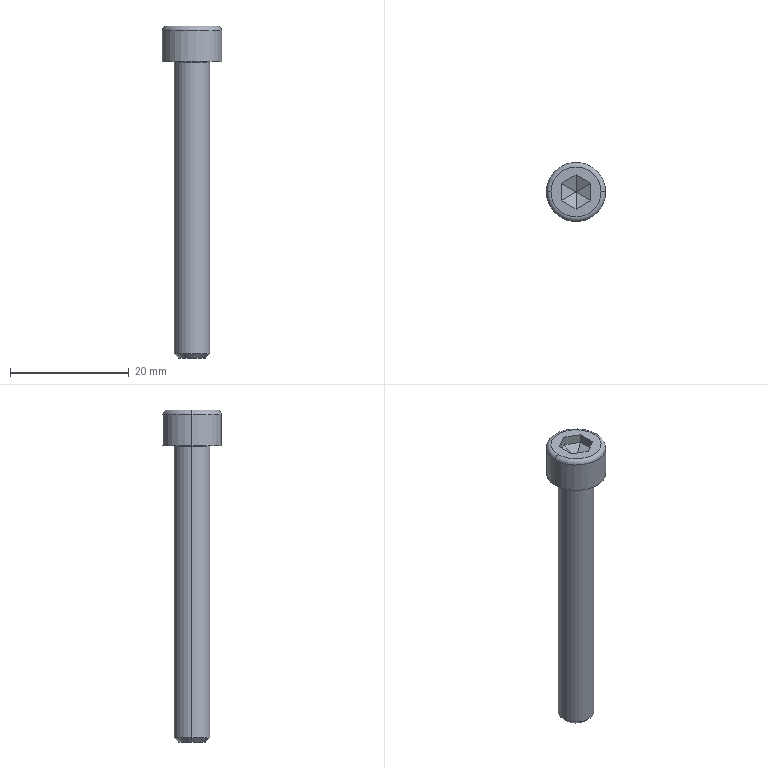Part | SolidWorks | features Chamfer 2, Fillet 2, ICE 2, Extrusion 1, RefAxis 1 | 1 solid | 26 faces | box 10 x 10 x 56 mm | volume 1832 mm3 | plane 16 | torus 4 | cylinder 4 | cone 2 | commonest cylinder face diameters 6 x2 10 x2
STEP:
#1=CARTESIAN_POINT('',(-3.1,0.,0.));
#2=VERTEX_POINT('',#1);
#3=CARTESIAN_POINT('',(3.1,0.,0.));
#4=VERTEX_POINT('',#3);
#5=CARTESIAN_POINT('',(0.,0.,0.));
#6=DIRECTION('',(0.,0.,1.));
#7=DIRECTION('',(1.,0.,0.));
#8=AXIS2_PLACEMENT_3D('',#5,#6,#7);
#9=CIRCLE('',#8,3.1);
#10=EDGE_CURVE('',#2,#4,#9,.T.);
#11=ORIENTED_EDGE('',*,*,#10,.F.);
#12=CARTESIAN_POINT('',(-3.,0.,-0.1));
#13=VERTEX_POINT('',#12);
#14=CARTESIAN_POINT('',(-3.1,0.,-0.1));
#15=DIRECTION('',(0.,1.,0.));
#16=DIRECTION('',(-1.,0.,0.));
#17=AXIS2_PLACEMENT_3D('',#14,#15,#16);
#18=CIRCLE('',#17,0.1);
#19=EDGE_CURVE('',#2,#13,#18,.T.);
#20=ORIENTED_EDGE('',*,*,#19,.T.);
#21=CARTESIAN_POINT('',(3.,0.,-0.1));
#22=VERTEX_POINT('',#21);
#23=CARTESIAN_POINT('',(0.,0.,-0.1));
#24=DIRECTION('',(0.,0.,-1.));
#25=DIRECTION('',(1.,0.,0.));
#26=AXIS2_PLACEMENT_3D('',#23,#24,#25);
#27=CIRCLE('',#26,3.);
#28=EDGE_CURVE('',#22,#13,#27,.T.);
#29=ORIENTED_EDGE('',*,*,#28,.F.);
#30=CARTESIAN_POINT('',(3.1,0.,-0.1));
#31=DIRECTION('',(0.,-1.,0.));
#32=DIRECTION('',(0.,0.,-1.));
#33=AXIS2_PLACEMENT_3D('',#30,#31,#32);
#34=CIRCLE('',#33,0.1);
#35=EDGE_CURVE('',#4,#22,#34,.T.);
#36=ORIENTED_EDGE('',*,*,#35,.F.);
#37=EDGE_LOOP('',(#11,#20,#29,#36));
#38=FACE_OUTER_BOUND('',#37,.T.);
#39=CARTESIAN_POINT('',(0.,0.,-0.1));
#40=DIRECTION('',(0.,0.,1.));
#41=DIRECTION('',(1.,0.,0.));
#42=AXIS2_PLACEMENT_3D('',#39,#40,#41);
#43=TOROIDAL_SURFACE('',#42,3.1,0.1);
#44=ADVANCED_FACE('',(#38),#43,.F.);
#45=CARTESIAN_POINT('',(-5.,0.,5.231));
#46=VERTEX_POINT('',#45);
#47=CARTESIAN_POINT('',(5.,0.,5.231));
#48=VERTEX_POINT('',#47);
#49=CARTESIAN_POINT('',(0.,0.,5.231));
#50=DIRECTION('',(0.,0.,-1.));
#51=DIRECTION('',(1.,0.,0.));
#52=AXIS2_PLACEMENT_3D('',#49,#50,#51);
#53=CIRCLE('',#52,5.);
#54=EDGE_CURVE('',#46,#48,#53,.T.);
#55=ORIENTED_EDGE('',*,*,#54,.F.);
#56=CARTESIAN_POINT('',(-4.231,0.,6.));
#57=VERTEX_POINT('',#56);
#58=CARTESIAN_POINT('',(-4.231,0.,5.231));
#59=DIRECTION('',(0.,1.,0.));
#60=DIRECTION('',(-1.,0.,0.));
#61=AXIS2_PLACEMENT_3D('',#58,#59,#60);
#62=CIRCLE('',#61,0.7692);
#63=EDGE_CURVE('',#46,#57,#62,.T.);
#64=ORIENTED_EDGE('',*,*,#63,.T.);
#65=CARTESIAN_POINT('',(4.231,0.,6.));
#66=VERTEX_POINT('',#65);
#67=CARTESIAN_POINT('',(0.,0.,6.));
#68=DIRECTION('',(0.,0.,1.));
#69=DIRECTION('',(1.,0.,0.));
#70=AXIS2_PLACEMENT_3D('',#67,#68,#69);
#71=CIRCLE('',#70,4.231);
#72=EDGE_CURVE('',#66,#57,#71,.T.);
#73=ORIENTED_EDGE('',*,*,#72,.F.);
#74=CARTESIAN_POINT('',(4.231,0.,5.231));
#75=DIRECTION('',(0.,-1.,0.));
#76=DIRECTION('',(0.,0.,-1.));
#77=AXIS2_PLACEMENT_3D('',#74,#75,#76);
#78=CIRCLE('',#77,0.7692);
#79=EDGE_CURVE('',#48,#66,#78,.T.);
#80=ORIENTED_EDGE('',*,*,#79,.F.);
#81=EDGE_LOOP('',(#55,#64,#73,#80));
#82=FACE_OUTER_BOUND('',#81,.T.);
#83=CARTESIAN_POINT('',(0.,0.,5.231));
#84=DIRECTION('',(0.,0.,1.));
#85=DIRECTION('',(1.,0.,0.));
#86=AXIS2_PLACEMENT_3D('',#83,#84,#85);
#87=TOROIDAL_SURFACE('',#86,4.231,0.7692);
#88=ADVANCED_FACE('',(#82),#87,.T.);
#89=CARTESIAN_POINT('',(-2.25,0.,-50.));
#90=VERTEX_POINT('',#89);
#91=CARTESIAN_POINT('',(2.25,0.,-50.));
#92=VERTEX_POINT('',#91);
#93=CARTESIAN_POINT('',(0.,0.,-50.));
#94=DIRECTION('',(0.,0.,-1.));
#95=DIRECTION('',(-1.,0.,0.));
#96=AXIS2_PLACEMENT_3D('',#93,#94,#95);
#97=CIRCLE('',#96,2.25);
#98=EDGE_CURVE('',#90,#92,#97,.T.);
#99=ORIENTED_EDGE('',*,*,#98,.F.);
#100=CARTESIAN_POINT('',(-3.,0.,-49.25));
#101=VERTEX_POINT('',#100);
#102=CARTESIAN_POINT('',(-2.25,0.,-50.));
#103=DIRECTION('',(-0.7071,0.,0.7071));
#104=VECTOR('',#103,1000.);
#105=LINE('',#102,#104);
#106=EDGE_CURVE('',#90,#101,#105,.T.);
#107=ORIENTED_EDGE('',*,*,#106,.T.);
#108=CARTESIAN_POINT('',(3.,0.,-49.25));
#109=VERTEX_POINT('',#108);
#110=CARTESIAN_POINT('',(0.,0.,-49.25));
#111=DIRECTION('',(0.,0.,1.));
#112=DIRECTION('',(-1.,0.,0.));
#113=AXIS2_PLACEMENT_3D('',#110,#111,#112);
#114=CIRCLE('',#113,3.);
#115=EDGE_CURVE('',#109,#101,#114,.T.);
#116=ORIENTED_EDGE('',*,*,#115,.F.);
#117=CARTESIAN_POINT('',(2.25,0.,-50.));
#118=DIRECTION('',(0.7071,0.,0.7071));
#119=VECTOR('',#118,1000.);
#120=LINE('',#117,#119);
#121=EDGE_CURVE('',#92,#109,#120,.T.);
#122=ORIENTED_EDGE('',*,*,#121,.F.);
#123=EDGE_LOOP('',(#99,#107,#116,#122));
#124=FACE_OUTER_BOUND('',#123,.T.);
#125=CARTESIAN_POINT('',(0.,0.,-50.));
#126=DIRECTION('',(0.,0.,1.));
#127=DIRECTION('',(1.,0.,0.));
#128=AXIS2_PLACEMENT_3D('',#125,#126,#127);
#129=CONICAL_SURFACE('',#128,2.25,0.7854);
#130=ADVANCED_FACE('',(#124),#129,.T.);
#131=ORIENTED_EDGE('',*,*,#115,.T.);
#132=CARTESIAN_POINT('',(-3.,0.,-50.));
#133=DIRECTION('',(0.,0.,1.));
#134=VECTOR('',#133,1000.);
#135=LINE('',#132,#134);
#136=EDGE_CURVE('',#101,#13,#135,.T.);
#137=ORIENTED_EDGE('',*,*,#136,.T.);
#138=CARTESIAN_POINT('',(0.,0.,-0.1));
#139=DIRECTION('',(0.,0.,-1.));
#140=DIRECTION('',(1.,0.,0.));
#141=AXIS2_PLACEMENT_3D('',#138,#139,#140);
#142=CIRCLE('',#141,3.);
#143=EDGE_CURVE('',#13,#22,#142,.T.);
#144=ORIENTED_EDGE('',*,*,#143,.T.);
#145=CARTESIAN_POINT('',(3.,0.,-50.));
#146=DIRECTION('',(0.,0.,1.));
#147=VECTOR('',#146,1000.);
#148=LINE('',#145,#147);
#149=EDGE_CURVE('',#109,#22,#148,.T.);
#150=ORIENTED_EDGE('',*,*,#149,.F.);
#151=EDGE_LOOP('',(#131,#137,#144,#150));
#152=FACE_OUTER_BOUND('',#151,.T.);
#153=CARTESIAN_POINT('',(0.,0.,-50.));
#154=DIRECTION('',(0.,0.,1.));
#155=DIRECTION('',(1.,0.,0.));
#156=AXIS2_PLACEMENT_3D('',#153,#154,#155);
#157=CYLINDRICAL_SURFACE('',#156,3.);
#158=ADVANCED_FACE('',(#152),#157,.T.);
#159=ORIENTED_EDGE('',*,*,#54,.T.);
#160=CARTESIAN_POINT('',(5.,0.,0.));
#161=VERTEX_POINT('',#160);
#162=CARTESIAN_POINT('',(5.,0.,6.));
#163=DIRECTION('',(0.,0.,-1.));
#164=VECTOR('',#163,1000.);
#165=LINE('',#162,#164);
#166=EDGE_CURVE('',#48,#161,#165,.T.);
#167=ORIENTED_EDGE('',*,*,#166,.T.);
#168=CARTESIAN_POINT('',(-5.,0.,0.));
#169=VERTEX_POINT('',#168);
#170=CARTESIAN_POINT('',(0.,0.,0.));
#171=DIRECTION('',(0.,0.,1.));
#172=DIRECTION('',(1.,0.,0.));
#173=AXIS2_PLACEMENT_3D('',#170,#171,#172);
#174=CIRCLE('',#173,5.);
#175=EDGE_CURVE('',#161,#169,#174,.T.);
#176=ORIENTED_EDGE('',*,*,#175,.T.);
#177=CARTESIAN_POINT('',(-5.,0.,6.));
#178=DIRECTION('',(0.,0.,-1.));
#179=VECTOR('',#178,1000.);
#180=LINE('',#177,#179);
#181=EDGE_CURVE('',#46,#169,#180,.T.);
#182=ORIENTED_EDGE('',*,*,#181,.F.);
#183=EDGE_LOOP('',(#159,#167,#176,#182));
#184=FACE_OUTER_BOUND('',#183,.T.);
#185=CARTESIAN_POINT('',(0.,0.,6.));
#186=DIRECTION('',(0.,0.,-1.));
#187=DIRECTION('',(-1.,0.,0.));
#188=AXIS2_PLACEMENT_3D('',#185,#186,#187);
#189=CYLINDRICAL_SURFACE('',#188,5.);
#190=ADVANCED_FACE('',(#184),#189,.T.);
#191=CARTESIAN_POINT('',(0.,0.,0.));
#192=DIRECTION('',(0.,0.,1.));
#193=DIRECTION('',(1.,0.,0.));
#194=AXIS2_PLACEMENT_3D('',#191,#192,#193);
#195=CIRCLE('',#194,3.1);
#196=EDGE_CURVE('',#4,#2,#195,.T.);
#197=ORIENTED_EDGE('',*,*,#196,.T.);
#198=ORIENTED_EDGE('',*,*,#10,.T.);
#199=EDGE_LOOP('',(#197,#198));
#200=FACE_BOUND('',#199,.T.);
#201=CARTESIAN_POINT('',(0.,0.,0.));
#202=DIRECTION('',(0.,0.,1.));
#203=DIRECTION('',(1.,0.,0.));
#204=AXIS2_PLACEMENT_3D('',#201,#202,#203);
#205=CIRCLE('',#204,5.);
#206=EDGE_CURVE('',#169,#161,#205,.T.);
#207=ORIENTED_EDGE('',*,*,#206,.F.);
#208=ORIENTED_EDGE('',*,*,#175,.F.);
#209=EDGE_LOOP('',(#207,#208));
#210=FACE_OUTER_BOUND('',#209,.T.);
#211=CARTESIAN_POINT('',(0.,0.,0.));
#212=DIRECTION('',(0.,0.,1.));
#213=DIRECTION('',(1.,0.,0.));
#214=AXIS2_PLACEMENT_3D('',#211,#212,#213);
#215=PLANE('',#214);
#216=ADVANCED_FACE('',(#200,#210),#215,.F.);
#217=ORIENTED_EDGE('',*,*,#166,.F.);
#218=CARTESIAN_POINT('',(0.,0.,5.231));
#219=DIRECTION('',(0.,0.,-1.));
#220=DIRECTION('',(1.,0.,0.));
#221=AXIS2_PLACEMENT_3D('',#218,#219,#220);
#222=CIRCLE('',#221,5.);
#223=EDGE_CURVE('',#48,#46,#222,.T.);
#224=ORIENTED_EDGE('',*,*,#223,.T.);
#225=ORIENTED_EDGE('',*,*,#181,.T.);
#226=ORIENTED_EDGE('',*,*,#206,.T.);
#227=EDGE_LOOP('',(#217,#224,#225,#226));
#228=FACE_OUTER_BOUND('',#227,.T.);
#229=CARTESIAN_POINT('',(0.,0.,6.));
#230=DIRECTION('',(0.,0.,-1.));
#231=DIRECTION('',(-1.,0.,0.));
#232=AXIS2_PLACEMENT_3D('',#229,#230,#231);
#233=CYLINDRICAL_SURFACE('',#232,5.);
#234=ADVANCED_FACE('',(#228),#233,.T.);
#235=ORIENTED_EDGE('',*,*,#72,.T.);
#236=CARTESIAN_POINT('',(0.,0.,6.));
#237=DIRECTION('',(0.,0.,1.));
#238=DIRECTION('',(1.,0.,0.));
#239=AXIS2_PLACEMENT_3D('',#236,#237,#238);
#240=CIRCLE('',#239,4.231);
#241=EDGE_CURVE('',#57,#66,#240,.T.);
#242=ORIENTED_EDGE('',*,*,#241,.T.);
#243=EDGE_LOOP('',(#235,#242));
#244=FACE_OUTER_BOUND('',#243,.T.);
#245=CARTESIAN_POINT('',(2.5,-1.443,6.));
#246=VERTEX_POINT('',#245);
#247=CARTESIAN_POINT('',(2.5,1.443,6.));
#248=VERTEX_POINT('',#247);
#249=CARTESIAN_POINT('',(2.5,-1.443,6.));
#250=DIRECTION('',(0.,1.,0.));
#251=VECTOR('',#250,1000.);
#252=LINE('',#249,#251);
#253=EDGE_CURVE('',#246,#248,#252,.T.);
#254=ORIENTED_EDGE('',*,*,#253,.F.);
#255=CARTESIAN_POINT('',(0.,-2.887,6.));
#256=VERTEX_POINT('',#255);
#257=CARTESIAN_POINT('',(0.,-2.887,6.));
#258=DIRECTION('',(0.866,0.5,0.));
#259=VECTOR('',#258,1000.);
#260=LINE('',#257,#259);
#261=EDGE_CURVE('',#256,#246,#260,.T.);
#262=ORIENTED_EDGE('',*,*,#261,.F.);
#263=CARTESIAN_POINT('',(-2.5,-1.443,6.));
#264=VERTEX_POINT('',#263);
#265=CARTESIAN_POINT('',(-2.5,-1.443,6.));
#266=DIRECTION('',(0.866,-0.5,0.));
#267=VECTOR('',#266,1000.);
#268=LINE('',#265,#267);
#269=EDGE_CURVE('',#264,#256,#268,.T.);
#270=ORIENTED_EDGE('',*,*,#269,.F.);
#271=CARTESIAN_POINT('',(-2.5,1.443,6.));
#272=VERTEX_POINT('',#271);
#273=CARTESIAN_POINT('',(-2.5,1.443,6.));
#274=DIRECTION('',(0.,-1.,0.));
#275=VECTOR('',#274,1000.);
#276=LINE('',#273,#275);
#277=EDGE_CURVE('',#272,#264,#276,.T.);
#278=ORIENTED_EDGE('',*,*,#277,.F.);
#279=CARTESIAN_POINT('',(0.,2.887,6.));
#280=VERTEX_POINT('',#279);
#281=CARTESIAN_POINT('',(0.,2.887,6.));
#282=DIRECTION('',(-0.866,-0.5,0.));
#283=VECTOR('',#282,1000.);
#284=LINE('',#281,#283);
#285=EDGE_CURVE('',#280,#272,#284,.T.);
#286=ORIENTED_EDGE('',*,*,#285,.F.);
#287=CARTESIAN_POINT('',(2.5,1.443,6.));
#288=DIRECTION('',(-0.866,0.5,0.));
#289=VECTOR('',#288,1000.);
#290=LINE('',#287,#289);
#291=EDGE_CURVE('',#248,#280,#290,.T.);
#292=ORIENTED_EDGE('',*,*,#291,.F.);
#293=EDGE_LOOP('',(#254,#262,#270,#278,#286,#292));
#294=FACE_BOUND('',#293,.T.);
#295=CARTESIAN_POINT('',(0.,0.,6.));
#296=DIRECTION('',(0.,0.,1.));
#297=DIRECTION('',(1.,0.,0.));
#298=AXIS2_PLACEMENT_3D('',#295,#296,#297);
#299=PLANE('',#298);
#300=ADVANCED_FACE('',(#244,#294),#299,.T.);
#301=CARTESIAN_POINT('',(2.5,1.443,4.441));
#302=VERTEX_POINT('',#301);
#303=CARTESIAN_POINT('',(2.5,1.443,3.));
#304=DIRECTION('',(0.,0.,1.));
#305=VECTOR('',#304,1000.);
#306=LINE('',#303,#305);
#307=EDGE_CURVE('',#302,#248,#306,.T.);
#308=ORIENTED_EDGE('',*,*,#307,.F.);
#309=CARTESIAN_POINT('',(2.5,-1.443,4.441));
#310=VERTEX_POINT('',#309);
#311=CARTESIAN_POINT('',(2.5,-1.443,4.441));
#312=DIRECTION('',(0.,-1.,0.));
#313=VECTOR('',#312,1000.);
#314=LINE('',#311,#313);
#315=EDGE_CURVE('',#302,#310,#314,.T.);
#316=ORIENTED_EDGE('',*,*,#315,.T.);
#317=CARTESIAN_POINT('',(2.5,-1.443,3.));
#318=DIRECTION('',(0.,0.,1.));
#319=VECTOR('',#318,1000.);
#320=LINE('',#317,#319);
#321=EDGE_CURVE('',#310,#246,#320,.T.);
#322=ORIENTED_EDGE('',*,*,#321,.T.);
#323=ORIENTED_EDGE('',*,*,#253,.T.);
#324=EDGE_LOOP('',(#308,#316,#322,#323));
#325=FACE_OUTER_BOUND('',#324,.T.);
#326=CARTESIAN_POINT('',(2.5,-1.443,3.));
#327=DIRECTION('',(1.,0.,0.));
#328=DIRECTION('',(0.,0.,-1.));
#329=AXIS2_PLACEMENT_3D('',#326,#327,#328);
#330=PLANE('',#329);
#331=ADVANCED_FACE('',(#325),#330,.F.);
#332=ORIENTED_EDGE('',*,*,#321,.F.);
#333=CARTESIAN_POINT('',(0.,-2.887,4.441));
#334=VERTEX_POINT('',#333);
#335=CARTESIAN_POINT('',(0.,-2.887,4.441));
#336=DIRECTION('',(-0.866,-0.5,0.));
#337=VECTOR('',#336,1000.);
#338=LINE('',#335,#337);
#339=EDGE_CURVE('',#310,#334,#338,.T.);
#340=ORIENTED_EDGE('',*,*,#339,.T.);
#341=CARTESIAN_POINT('',(0.,-2.887,3.));
#342=DIRECTION('',(0.,0.,1.));
#343=VECTOR('',#342,1000.);
#344=LINE('',#341,#343);
#345=EDGE_CURVE('',#334,#256,#344,.T.);
#346=ORIENTED_EDGE('',*,*,#345,.T.);
#347=ORIENTED_EDGE('',*,*,#261,.T.);
#348=EDGE_LOOP('',(#332,#340,#346,#347));
#349=FACE_OUTER_BOUND('',#348,.T.);
#350=CARTESIAN_POINT('',(0.,-2.887,3.));
#351=DIRECTION('',(0.5,-0.866,0.));
#352=DIRECTION('',(0.866,0.5,0.));
#353=AXIS2_PLACEMENT_3D('',#350,#351,#352);
#354=PLANE('',#353);
#355=ADVANCED_FACE('',(#349),#354,.F.);
#356=ORIENTED_EDGE('',*,*,#345,.F.);
#357=CARTESIAN_POINT('',(-2.5,-1.443,4.441));
#358=VERTEX_POINT('',#357);
#359=CARTESIAN_POINT('',(-2.5,-1.443,4.441));
#360=DIRECTION('',(-0.866,0.5,0.));
#361=VECTOR('',#360,1000.);
#362=LINE('',#359,#361);
#363=EDGE_CURVE('',#334,#358,#362,.T.);
#364=ORIENTED_EDGE('',*,*,#363,.T.);
#365=CARTESIAN_POINT('',(-2.5,-1.443,3.));
#366=DIRECTION('',(0.,0.,1.));
#367=VECTOR('',#366,1000.);
#368=LINE('',#365,#367);
#369=EDGE_CURVE('',#358,#264,#368,.T.);
#370=ORIENTED_EDGE('',*,*,#369,.T.);
#371=ORIENTED_EDGE('',*,*,#269,.T.);
#372=EDGE_LOOP('',(#356,#364,#370,#371));
#373=FACE_OUTER_BOUND('',#372,.T.);
#374=CARTESIAN_POINT('',(-2.5,-1.443,3.));
#375=DIRECTION('',(-0.5,-0.866,0.));
#376=DIRECTION('',(0.866,-0.5,0.));
#377=AXIS2_PLACEMENT_3D('',#374,#375,#376);
#378=PLANE('',#377);
#379=ADVANCED_FACE('',(#373),#378,.F.);
#380=ORIENTED_EDGE('',*,*,#369,.F.);
#381=CARTESIAN_POINT('',(-2.5,1.443,4.441));
#382=VERTEX_POINT('',#381);
#383=CARTESIAN_POINT('',(-2.5,1.443,4.441));
#384=DIRECTION('',(0.,1.,0.));
#385=VECTOR('',#384,1000.);
#386=LINE('',#383,#385);
#387=EDGE_CURVE('',#358,#382,#386,.T.);
#388=ORIENTED_EDGE('',*,*,#387,.T.);
#389=CARTESIAN_POINT('',(-2.5,1.443,3.));
#390=DIRECTION('',(0.,0.,1.));
#391=VECTOR('',#390,1000.);
#392=LINE('',#389,#391);
#393=EDGE_CURVE('',#382,#272,#392,.T.);
#394=ORIENTED_EDGE('',*,*,#393,.T.);
#395=ORIENTED_EDGE('',*,*,#277,.T.);
#396=EDGE_LOOP('',(#380,#388,#394,#395));
#397=FACE_OUTER_BOUND('',#396,.T.);
#398=CARTESIAN_POINT('',(-2.5,1.443,3.));
#399=DIRECTION('',(-1.,0.,0.));
#400=DIRECTION('',(0.,0.,1.));
#401=AXIS2_PLACEMENT_3D('',#398,#399,#400);
#402=PLANE('',#401);
#403=ADVANCED_FACE('',(#397),#402,.F.);
#404=ORIENTED_EDGE('',*,*,#393,.F.);
#405=CARTESIAN_POINT('',(0.,2.887,4.441));
#406=VERTEX_POINT('',#405);
#407=CARTESIAN_POINT('',(0.,2.887,4.441));
#408=DIRECTION('',(0.866,0.5,0.));
#409=VECTOR('',#408,1000.);
#410=LINE('',#407,#409);
#411=EDGE_CURVE('',#382,#406,#410,.T.);
#412=ORIENTED_EDGE('',*,*,#411,.T.);
#413=CARTESIAN_POINT('',(0.,2.887,3.));
#414=DIRECTION('',(0.,0.,1.));
#415=VECTOR('',#414,1000.);
#416=LINE('',#413,#415);
#417=EDGE_CURVE('',#406,#280,#416,.T.);
#418=ORIENTED_EDGE('',*,*,#417,.T.);
#419=ORIENTED_EDGE('',*,*,#285,.T.);
#420=EDGE_LOOP('',(#404,#412,#418,#419));
#421=FACE_OUTER_BOUND('',#420,.T.);
#422=CARTESIAN_POINT('',(0.,2.887,3.));
#423=DIRECTION('',(-0.5,0.866,0.));
#424=DIRECTION('',(-0.866,-0.5,0.));
#425=AXIS2_PLACEMENT_3D('',#422,#423,#424);
#426=PLANE('',#425);
#427=ADVANCED_FACE('',(#421),#426,.F.);
#428=ORIENTED_EDGE('',*,*,#417,.F.);
#429=CARTESIAN_POINT('',(2.5,1.443,4.441));
#430=DIRECTION('',(0.866,-0.5,0.));
#431=VECTOR('',#430,1000.);
#432=LINE('',#429,#431);
#433=EDGE_CURVE('',#406,#302,#432,.T.);
#434=ORIENTED_EDGE('',*,*,#433,.T.);
#435=ORIENTED_EDGE('',*,*,#307,.T.);
#436=ORIENTED_EDGE('',*,*,#291,.T.);
#437=EDGE_LOOP('',(#428,#434,#435,#436));
#438=FACE_OUTER_BOUND('',#437,.T.);
#439=CARTESIAN_POINT('',(2.5,1.443,3.));
#440=DIRECTION('',(0.5,0.866,0.));
#441=DIRECTION('',(-0.866,0.5,0.));
#442=AXIS2_PLACEMENT_3D('',#439,#440,#441);
#443=PLANE('',#442);
#444=ADVANCED_FACE('',(#438),#443,.F.);
#445=CARTESIAN_POINT('',(0.,0.004907,3.));
#446=VERTEX_POINT('',#445);
#447=CARTESIAN_POINT('',(-0.00425,0.002453,3.));
#448=VERTEX_POINT('',#447);
#449=CARTESIAN_POINT('',(-0.002125,0.00368,3.));
#450=DIRECTION('',(-0.866,-0.5,0.));
#451=VECTOR('',#450,1000.);
#452=LINE('',#449,#451);
#453=EDGE_CURVE('',#446,#448,#452,.T.);
#454=ORIENTED_EDGE('',*,*,#453,.T.);
#455=CARTESIAN_POINT('',(-0.00425,-0.002453,3.));
#456=VERTEX_POINT('',#455);
#457=CARTESIAN_POINT('',(-0.00425,0.,3.));
#458=DIRECTION('',(0.,-1.,0.));
#459=VECTOR('',#458,1000.);
#460=LINE('',#457,#459);
#461=EDGE_CURVE('',#448,#456,#460,.T.);
#462=ORIENTED_EDGE('',*,*,#461,.T.);
#463=CARTESIAN_POINT('',(0.,-0.004907,3.));
#464=VERTEX_POINT('',#463);
#465=CARTESIAN_POINT('',(-0.002125,-0.00368,3.));
#466=DIRECTION('',(0.866,-0.5,0.));
#467=VECTOR('',#466,1000.);
#468=LINE('',#465,#467);
#469=EDGE_CURVE('',#456,#464,#468,.T.);
#470=ORIENTED_EDGE('',*,*,#469,.T.);
#471=CARTESIAN_POINT('',(0.00425,-0.002453,3.));
#472=VERTEX_POINT('',#471);
#473=CARTESIAN_POINT('',(0.002125,-0.00368,3.));
#474=DIRECTION('',(0.866,0.5,0.));
#475=VECTOR('',#474,1000.);
#476=LINE('',#473,#475);
#477=EDGE_CURVE('',#464,#472,#476,.T.);
#478=ORIENTED_EDGE('',*,*,#477,.T.);
#479=CARTESIAN_POINT('',(0.00425,0.002453,3.));
#480=VERTEX_POINT('',#479);
#481=CARTESIAN_POINT('',(0.00425,0.,3.));
#482=DIRECTION('',(0.,1.,0.));
#483=VECTOR('',#482,1000.);
#484=LINE('',#481,#483);
#485=EDGE_CURVE('',#472,#480,#484,.T.);
#486=ORIENTED_EDGE('',*,*,#485,.T.);
#487=CARTESIAN_POINT('',(0.002125,0.00368,3.));
#488=DIRECTION('',(-0.866,0.5,0.));
#489=VECTOR('',#488,1000.);
#490=LINE('',#487,#489);
#491=EDGE_CURVE('',#480,#446,#490,.T.);
#492=ORIENTED_EDGE('',*,*,#491,.T.);
#493=EDGE_LOOP('',(#454,#462,#470,#478,#486,#492));
#494=FACE_OUTER_BOUND('',#493,.T.);
#495=CARTESIAN_POINT('',(0.,0.,3.));
#496=DIRECTION('',(0.,0.,1.));
#497=DIRECTION('',(1.,0.,0.));
#498=AXIS2_PLACEMENT_3D('',#495,#496,#497);
#499=PLANE('',#498);
#500=ADVANCED_FACE('',(#494),#499,.T.);
#501=ORIENTED_EDGE('',*,*,#136,.F.);
#502=CARTESIAN_POINT('',(0.,0.,-49.25));
#503=DIRECTION('',(0.,0.,1.));
#504=DIRECTION('',(-1.,0.,0.));
#505=AXIS2_PLACEMENT_3D('',#502,#503,#504);
#506=CIRCLE('',#505,3.);
#507=EDGE_CURVE('',#101,#109,#506,.T.);
#508=ORIENTED_EDGE('',*,*,#507,.T.);
#509=ORIENTED_EDGE('',*,*,#149,.T.);
#510=ORIENTED_EDGE('',*,*,#28,.T.);
#511=EDGE_LOOP('',(#501,#508,#509,#510));
#512=FACE_OUTER_BOUND('',#511,.T.);
#513=CARTESIAN_POINT('',(0.,0.,-50.));
#514=DIRECTION('',(0.,0.,1.));
#515=DIRECTION('',(1.,0.,0.));
#516=AXIS2_PLACEMENT_3D('',#513,#514,#515);
#517=CYLINDRICAL_SURFACE('',#516,3.);
#518=ADVANCED_FACE('',(#512),#517,.T.);
#519=CARTESIAN_POINT('',(0.,0.,-50.));
#520=DIRECTION('',(0.,0.,-1.));
#521=DIRECTION('',(-1.,0.,0.));
#522=AXIS2_PLACEMENT_3D('',#519,#520,#521);
#523=CIRCLE('',#522,2.25);
#524=EDGE_CURVE('',#92,#90,#523,.T.);
#525=ORIENTED_EDGE('',*,*,#524,.T.);
#526=ORIENTED_EDGE('',*,*,#98,.T.);
#527=EDGE_LOOP('',(#525,#526));
#528=FACE_OUTER_BOUND('',#527,.T.);
#529=CARTESIAN_POINT('',(0.,0.,-50.));
#530=DIRECTION('',(0.,0.,-1.));
#531=DIRECTION('',(-1.,0.,0.));
#532=AXIS2_PLACEMENT_3D('',#529,#530,#531);
#533=PLANE('',#532);
#534=ADVANCED_FACE('',(#528),#533,.T.);
#535=ORIENTED_EDGE('',*,*,#106,.F.);
#536=ORIENTED_EDGE('',*,*,#524,.F.);
#537=ORIENTED_EDGE('',*,*,#121,.T.);
#538=ORIENTED_EDGE('',*,*,#507,.F.);
#539=EDGE_LOOP('',(#535,#536,#537,#538));
#540=FACE_OUTER_BOUND('',#539,.T.);
#541=CARTESIAN_POINT('',(0.,0.,-50.));
#542=DIRECTION('',(0.,0.,1.));
#543=DIRECTION('',(1.,0.,0.));
#544=AXIS2_PLACEMENT_3D('',#541,#542,#543);
#545=CONICAL_SURFACE('',#544,2.25,0.7854);
#546=ADVANCED_FACE('',(#540),#545,.T.);
#547=ORIENTED_EDGE('',*,*,#63,.F.);
#548=ORIENTED_EDGE('',*,*,#223,.F.);
#549=ORIENTED_EDGE('',*,*,#79,.T.);
#550=ORIENTED_EDGE('',*,*,#241,.F.);
#551=EDGE_LOOP('',(#547,#548,#549,#550));
#552=FACE_OUTER_BOUND('',#551,.T.);
#553=CARTESIAN_POINT('',(0.,0.,5.231));
#554=DIRECTION('',(0.,0.,1.));
#555=DIRECTION('',(1.,0.,0.));
#556=AXIS2_PLACEMENT_3D('',#553,#554,#555);
#557=TOROIDAL_SURFACE('',#556,4.231,0.7692);
#558=ADVANCED_FACE('',(#552),#557,.T.);
#559=CARTESIAN_POINT('',(0.0034,-0.001963,3.));
#560=DIRECTION('',(-0.7746,0.4472,-0.4472));
#561=VECTOR('',#560,1000.);
#562=LINE('',#559,#561);
#563=EDGE_CURVE('',#310,#472,#562,.T.);
#564=ORIENTED_EDGE('',*,*,#563,.F.);
#565=ORIENTED_EDGE('',*,*,#315,.F.);
#566=CARTESIAN_POINT('',(0.0034,0.001963,3.));
#567=DIRECTION('',(0.7746,0.4472,0.4472));
#568=VECTOR('',#567,1000.);
#569=LINE('',#566,#568);
#570=EDGE_CURVE('',#480,#302,#569,.T.);
#571=ORIENTED_EDGE('',*,*,#570,.F.);
#572=ORIENTED_EDGE('',*,*,#485,.F.);
#573=EDGE_LOOP('',(#564,#565,#571,#572));
#574=FACE_OUTER_BOUND('',#573,.T.);
#575=CARTESIAN_POINT('',(0.00425,0.,3.));
#576=DIRECTION('',(0.5,0.,-0.866));
#577=DIRECTION('',(0.,1.,0.));
#578=AXIS2_PLACEMENT_3D('',#575,#576,#577);
#579=PLANE('',#578);
#580=ADVANCED_FACE('',(#574),#579,.F.);
#581=ORIENTED_EDGE('',*,*,#570,.T.);
#582=ORIENTED_EDGE('',*,*,#433,.F.);
#583=CARTESIAN_POINT('',(0.,0.003926,3.));
#584=DIRECTION('',(0.,0.8944,0.4472));
#585=VECTOR('',#584,1000.);
#586=LINE('',#583,#585);
#587=EDGE_CURVE('',#446,#406,#586,.T.);
#588=ORIENTED_EDGE('',*,*,#587,.F.);
#589=ORIENTED_EDGE('',*,*,#491,.F.);
#590=EDGE_LOOP('',(#581,#582,#588,#589));
#591=FACE_OUTER_BOUND('',#590,.T.);
#592=CARTESIAN_POINT('',(0.002125,0.00368,3.));
#593=DIRECTION('',(0.25,0.433,-0.866));
#594=DIRECTION('',(-0.866,0.5,0.));
#595=AXIS2_PLACEMENT_3D('',#592,#593,#594);
#596=PLANE('',#595);
#597=ADVANCED_FACE('',(#591),#596,.F.);
#598=ORIENTED_EDGE('',*,*,#563,.T.);
#599=ORIENTED_EDGE('',*,*,#477,.F.);
#600=CARTESIAN_POINT('',(0.,-0.003926,3.));
#601=DIRECTION('',(0.,0.8944,-0.4472));
#602=VECTOR('',#601,1000.);
#603=LINE('',#600,#602);
#604=EDGE_CURVE('',#334,#464,#603,.T.);
#605=ORIENTED_EDGE('',*,*,#604,.F.);
#606=ORIENTED_EDGE('',*,*,#339,.F.);
#607=EDGE_LOOP('',(#598,#599,#605,#606));
#608=FACE_OUTER_BOUND('',#607,.T.);
#609=CARTESIAN_POINT('',(0.002125,-0.00368,3.));
#610=DIRECTION('',(0.25,-0.433,-0.866));
#611=DIRECTION('',(0.866,0.5,0.));
#612=AXIS2_PLACEMENT_3D('',#609,#610,#611);
#613=PLANE('',#612);
#614=ADVANCED_FACE('',(#608),#613,.F.);
#615=ORIENTED_EDGE('',*,*,#587,.T.);
#616=ORIENTED_EDGE('',*,*,#411,.F.);
#617=CARTESIAN_POINT('',(-0.0034,0.001963,3.));
#618=DIRECTION('',(-0.7746,0.4472,0.4472));
#619=VECTOR('',#618,1000.);
#620=LINE('',#617,#619);
#621=EDGE_CURVE('',#448,#382,#620,.T.);
#622=ORIENTED_EDGE('',*,*,#621,.F.);
#623=ORIENTED_EDGE('',*,*,#453,.F.);
#624=EDGE_LOOP('',(#615,#616,#622,#623));
#625=FACE_OUTER_BOUND('',#624,.T.);
#626=CARTESIAN_POINT('',(-0.002125,0.00368,3.));
#627=DIRECTION('',(-0.25,0.433,-0.866));
#628=DIRECTION('',(-0.866,-0.5,0.));
#629=AXIS2_PLACEMENT_3D('',#626,#627,#628);
#630=PLANE('',#629);
#631=ADVANCED_FACE('',(#625),#630,.F.);
#632=ORIENTED_EDGE('',*,*,#604,.T.);
#633=ORIENTED_EDGE('',*,*,#469,.F.);
#634=CARTESIAN_POINT('',(-0.0034,-0.001963,3.));
#635=DIRECTION('',(0.7746,0.4472,-0.4472));
#636=VECTOR('',#635,1000.);
#637=LINE('',#634,#636);
#638=EDGE_CURVE('',#358,#456,#637,.T.);
#639=ORIENTED_EDGE('',*,*,#638,.F.);
#640=ORIENTED_EDGE('',*,*,#363,.F.);
#641=EDGE_LOOP('',(#632,#633,#639,#640));
#642=FACE_OUTER_BOUND('',#641,.T.);
#643=CARTESIAN_POINT('',(-0.002125,-0.00368,3.));
#644=DIRECTION('',(-0.25,-0.433,-0.866));
#645=DIRECTION('',(0.866,-0.5,0.));
#646=AXIS2_PLACEMENT_3D('',#643,#644,#645);
#647=PLANE('',#646);
#648=ADVANCED_FACE('',(#642),#647,.F.);
#649=ORIENTED_EDGE('',*,*,#621,.T.);
#650=ORIENTED_EDGE('',*,*,#387,.F.);
#651=ORIENTED_EDGE('',*,*,#638,.T.);
#652=ORIENTED_EDGE('',*,*,#461,.F.);
#653=EDGE_LOOP('',(#649,#650,#651,#652));
#654=FACE_OUTER_BOUND('',#653,.T.);
#655=CARTESIAN_POINT('',(-0.00425,0.,3.));
#656=DIRECTION('',(-0.5,0.,-0.866));
#657=DIRECTION('',(0.,-1.,0.));
#658=AXIS2_PLACEMENT_3D('',#655,#656,#657);
#659=PLANE('',#658);
#660=ADVANCED_FACE('',(#654),#659,.F.);
#661=ORIENTED_EDGE('',*,*,#19,.F.);
#662=ORIENTED_EDGE('',*,*,#196,.F.);
#663=ORIENTED_EDGE('',*,*,#35,.T.);
#664=ORIENTED_EDGE('',*,*,#143,.F.);
#665=EDGE_LOOP('',(#661,#662,#663,#664));
#666=FACE_OUTER_BOUND('',#665,.T.);
#667=CARTESIAN_POINT('',(0.,0.,-0.1));
#668=DIRECTION('',(0.,0.,1.));
#669=DIRECTION('',(1.,0.,0.));
#670=AXIS2_PLACEMENT_3D('',#667,#668,#669);
#671=TOROIDAL_SURFACE('',#670,3.1,0.1);
#672=ADVANCED_FACE('',(#666),#671,.F.);
#673=CLOSED_SHELL('',(#44,#88,#130,#158,#190,#216,#234,#300,#331,#355,#379,#403,#427,#444,#500,#518,#534,#546,#558,#580,#597,#614,#631,#648,#660,#672));
#674=MANIFOLD_SOLID_BREP('',#673);
#675=CARTESIAN_POINT('',(0.,0.,0.));
#676=DIRECTION('',(0.,0.,1.));
#677=DIRECTION('',(1.,0.,0.));
#678=AXIS2_PLACEMENT_3D('',#675,#676,#677);
#679=(LENGTH_UNIT()NAMED_UNIT(*)SI_UNIT(.MILLI.,.METRE.));
#680=UNCERTAINTY_MEASURE_WITH_UNIT(LENGTH_MEASURE(0.00001),#679,'','');
#681=(NAMED_UNIT(*)PLANE_ANGLE_UNIT()SI_UNIT($,.RADIAN.));
#682=(NAMED_UNIT(*)SI_UNIT($,.STERADIAN.)SOLID_ANGLE_UNIT());
#683=(GEOMETRIC_REPRESENTATION_CONTEXT(3)GLOBAL_UNCERTAINTY_ASSIGNED_CONTEXT((#680))GLOBAL_UNIT_ASSIGNED_CONTEXT((#679,#681,#682))REPRESENTATION_CONTEXT('',''));
#684=ADVANCED_BREP_SHAPE_REPRESENTATION('',(#674,#678),#683);